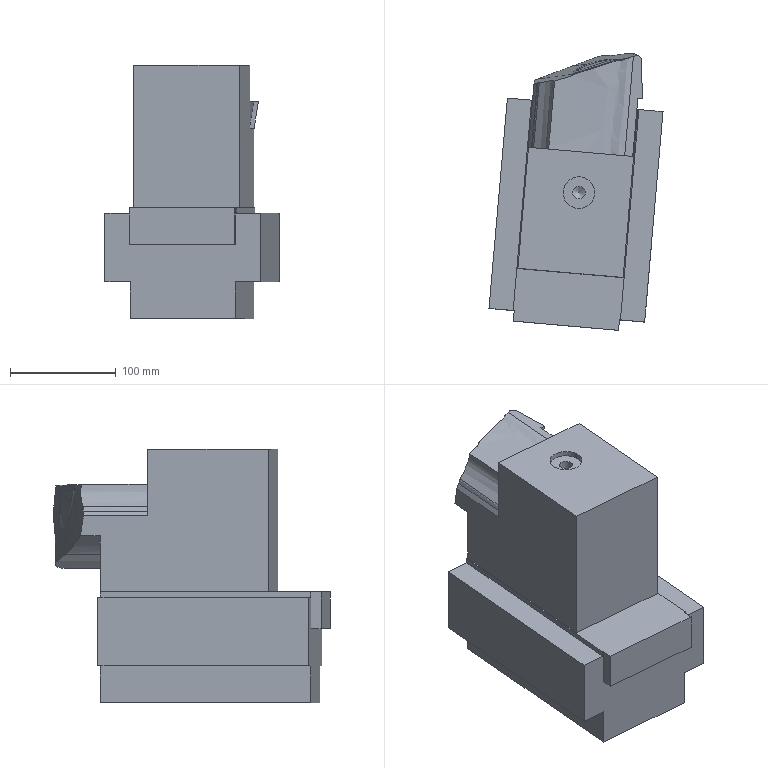Part | NX | features solid 2 | 1 solid | 89 faces | box 164.868 x 261.973 x 240 mm | volume 4872960 mm3 | spline 48 | plane 31 | cylinder 9 | cone 1 | commonest cylinder face diameters 20 x4 60 x2 12 x1 26 x1 30 x1